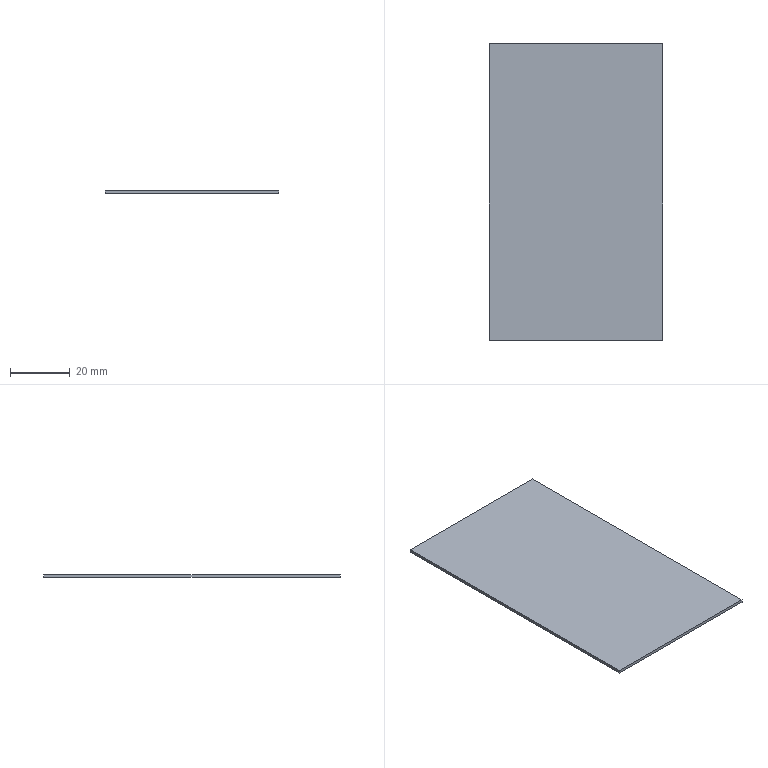Part | SolidWorks | features Extrusion 1 | 1 solid | 6 faces | box 58 x 99 x 1 mm | volume 5742 mm3 | plane 6
STEP:
#1=CARTESIAN_POINT('',(29.,-49.5,0.));
#2=VERTEX_POINT('',#1);
#3=CARTESIAN_POINT('',(29.,49.5,0.));
#4=VERTEX_POINT('',#3);
#5=CARTESIAN_POINT('',(29.,49.5,0.));
#6=DIRECTION('',(0.,1.,0.));
#7=VECTOR('',#6,1000.);
#8=LINE('',#5,#7);
#9=EDGE_CURVE('',#2,#4,#8,.T.);
#10=ORIENTED_EDGE('',*,*,#9,.T.);
#11=CARTESIAN_POINT('',(29.,49.5,1.));
#12=VERTEX_POINT('',#11);
#13=CARTESIAN_POINT('',(29.,49.5,1.));
#14=DIRECTION('',(0.,0.,-1.));
#15=VECTOR('',#14,1000.);
#16=LINE('',#13,#15);
#17=EDGE_CURVE('',#12,#4,#16,.T.);
#18=ORIENTED_EDGE('',*,*,#17,.F.);
#19=CARTESIAN_POINT('',(29.,-49.5,1.));
#20=VERTEX_POINT('',#19);
#21=CARTESIAN_POINT('',(29.,49.5,1.));
#22=DIRECTION('',(0.,1.,0.));
#23=VECTOR('',#22,1000.);
#24=LINE('',#21,#23);
#25=EDGE_CURVE('',#20,#12,#24,.T.);
#26=ORIENTED_EDGE('',*,*,#25,.F.);
#27=CARTESIAN_POINT('',(29.,-49.5,1.));
#28=DIRECTION('',(0.,0.,-1.));
#29=VECTOR('',#28,1000.);
#30=LINE('',#27,#29);
#31=EDGE_CURVE('',#20,#2,#30,.T.);
#32=ORIENTED_EDGE('',*,*,#31,.T.);
#33=EDGE_LOOP('',(#10,#18,#26,#32));
#34=FACE_OUTER_BOUND('',#33,.T.);
#35=CARTESIAN_POINT('',(29.,49.5,1.));
#36=DIRECTION('',(-1.,0.,0.));
#37=DIRECTION('',(0.,-1.,0.));
#38=AXIS2_PLACEMENT_3D('',#35,#36,#37);
#39=PLANE('',#38);
#40=ADVANCED_FACE('',(#34),#39,.F.);
#41=CARTESIAN_POINT('',(-29.,49.5,0.));
#42=VERTEX_POINT('',#41);
#43=CARTESIAN_POINT('',(-29.,49.5,0.));
#44=DIRECTION('',(-1.,0.,0.));
#45=VECTOR('',#44,1000.);
#46=LINE('',#43,#45);
#47=EDGE_CURVE('',#4,#42,#46,.T.);
#48=ORIENTED_EDGE('',*,*,#47,.T.);
#49=CARTESIAN_POINT('',(-29.,49.5,1.));
#50=VERTEX_POINT('',#49);
#51=CARTESIAN_POINT('',(-29.,49.5,1.));
#52=DIRECTION('',(0.,0.,-1.));
#53=VECTOR('',#52,1000.);
#54=LINE('',#51,#53);
#55=EDGE_CURVE('',#50,#42,#54,.T.);
#56=ORIENTED_EDGE('',*,*,#55,.F.);
#57=CARTESIAN_POINT('',(-29.,49.5,1.));
#58=DIRECTION('',(-1.,0.,0.));
#59=VECTOR('',#58,1000.);
#60=LINE('',#57,#59);
#61=EDGE_CURVE('',#12,#50,#60,.T.);
#62=ORIENTED_EDGE('',*,*,#61,.F.);
#63=ORIENTED_EDGE('',*,*,#17,.T.);
#64=EDGE_LOOP('',(#48,#56,#62,#63));
#65=FACE_OUTER_BOUND('',#64,.T.);
#66=CARTESIAN_POINT('',(-29.,49.5,1.));
#67=DIRECTION('',(0.,-1.,0.));
#68=DIRECTION('',(0.,0.,-1.));
#69=AXIS2_PLACEMENT_3D('',#66,#67,#68);
#70=PLANE('',#69);
#71=ADVANCED_FACE('',(#65),#70,.F.);
#72=CARTESIAN_POINT('',(-29.,-49.5,0.));
#73=VERTEX_POINT('',#72);
#74=CARTESIAN_POINT('',(-29.,49.5,0.));
#75=DIRECTION('',(0.,-1.,0.));
#76=VECTOR('',#75,1000.);
#77=LINE('',#74,#76);
#78=EDGE_CURVE('',#42,#73,#77,.T.);
#79=ORIENTED_EDGE('',*,*,#78,.T.);
#80=CARTESIAN_POINT('',(-29.,-49.5,1.));
#81=VERTEX_POINT('',#80);
#82=CARTESIAN_POINT('',(-29.,-49.5,1.));
#83=DIRECTION('',(0.,0.,-1.));
#84=VECTOR('',#83,1000.);
#85=LINE('',#82,#84);
#86=EDGE_CURVE('',#81,#73,#85,.T.);
#87=ORIENTED_EDGE('',*,*,#86,.F.);
#88=CARTESIAN_POINT('',(-29.,49.5,1.));
#89=DIRECTION('',(0.,-1.,0.));
#90=VECTOR('',#89,1000.);
#91=LINE('',#88,#90);
#92=EDGE_CURVE('',#50,#81,#91,.T.);
#93=ORIENTED_EDGE('',*,*,#92,.F.);
#94=ORIENTED_EDGE('',*,*,#55,.T.);
#95=EDGE_LOOP('',(#79,#87,#93,#94));
#96=FACE_OUTER_BOUND('',#95,.T.);
#97=CARTESIAN_POINT('',(-29.,49.5,1.));
#98=DIRECTION('',(1.,0.,0.));
#99=DIRECTION('',(0.,1.,0.));
#100=AXIS2_PLACEMENT_3D('',#97,#98,#99);
#101=PLANE('',#100);
#102=ADVANCED_FACE('',(#96),#101,.F.);
#103=CARTESIAN_POINT('',(-29.,-49.5,0.));
#104=DIRECTION('',(1.,0.,0.));
#105=VECTOR('',#104,1000.);
#106=LINE('',#103,#105);
#107=EDGE_CURVE('',#73,#2,#106,.T.);
#108=ORIENTED_EDGE('',*,*,#107,.T.);
#109=ORIENTED_EDGE('',*,*,#31,.F.);
#110=CARTESIAN_POINT('',(-29.,-49.5,1.));
#111=DIRECTION('',(1.,0.,0.));
#112=VECTOR('',#111,1000.);
#113=LINE('',#110,#112);
#114=EDGE_CURVE('',#81,#20,#113,.T.);
#115=ORIENTED_EDGE('',*,*,#114,.F.);
#116=ORIENTED_EDGE('',*,*,#86,.T.);
#117=EDGE_LOOP('',(#108,#109,#115,#116));
#118=FACE_OUTER_BOUND('',#117,.T.);
#119=CARTESIAN_POINT('',(-29.,-49.5,1.));
#120=DIRECTION('',(0.,1.,0.));
#121=DIRECTION('',(0.,0.,1.));
#122=AXIS2_PLACEMENT_3D('',#119,#120,#121);
#123=PLANE('',#122);
#124=ADVANCED_FACE('',(#118),#123,.F.);
#125=ORIENTED_EDGE('',*,*,#25,.T.);
#126=ORIENTED_EDGE('',*,*,#61,.T.);
#127=ORIENTED_EDGE('',*,*,#92,.T.);
#128=ORIENTED_EDGE('',*,*,#114,.T.);
#129=EDGE_LOOP('',(#125,#126,#127,#128));
#130=FACE_OUTER_BOUND('',#129,.T.);
#131=CARTESIAN_POINT('',(0.,0.,1.));
#132=DIRECTION('',(0.,0.,1.));
#133=DIRECTION('',(1.,0.,0.));
#134=AXIS2_PLACEMENT_3D('',#131,#132,#133);
#135=PLANE('',#134);
#136=ADVANCED_FACE('',(#130),#135,.T.);
#137=ORIENTED_EDGE('',*,*,#9,.F.);
#138=ORIENTED_EDGE('',*,*,#107,.F.);
#139=ORIENTED_EDGE('',*,*,#78,.F.);
#140=ORIENTED_EDGE('',*,*,#47,.F.);
#141=EDGE_LOOP('',(#137,#138,#139,#140));
#142=FACE_OUTER_BOUND('',#141,.T.);
#143=CARTESIAN_POINT('',(0.,0.,0.));
#144=DIRECTION('',(0.,0.,1.));
#145=DIRECTION('',(1.,0.,0.));
#146=AXIS2_PLACEMENT_3D('',#143,#144,#145);
#147=PLANE('',#146);
#148=ADVANCED_FACE('',(#142),#147,.F.);
#149=CLOSED_SHELL('',(#40,#71,#102,#124,#136,#148));
#150=MANIFOLD_SOLID_BREP('',#149);
#151=CARTESIAN_POINT('',(0.,0.,0.));
#152=DIRECTION('',(0.,0.,1.));
#153=DIRECTION('',(1.,0.,0.));
#154=AXIS2_PLACEMENT_3D('',#151,#152,#153);
#155=(LENGTH_UNIT()NAMED_UNIT(*)SI_UNIT(.MILLI.,.METRE.));
#156=UNCERTAINTY_MEASURE_WITH_UNIT(LENGTH_MEASURE(0.00001),#155,'','');
#157=(NAMED_UNIT(*)PLANE_ANGLE_UNIT()SI_UNIT($,.RADIAN.));
#158=(NAMED_UNIT(*)SI_UNIT($,.STERADIAN.)SOLID_ANGLE_UNIT());
#159=(GEOMETRIC_REPRESENTATION_CONTEXT(3)GLOBAL_UNCERTAINTY_ASSIGNED_CONTEXT((#156))GLOBAL_UNIT_ASSIGNED_CONTEXT((#155,#157,#158))REPRESENTATION_CONTEXT('',''));
#160=ADVANCED_BREP_SHAPE_REPRESENTATION('',(#150,#154),#159);